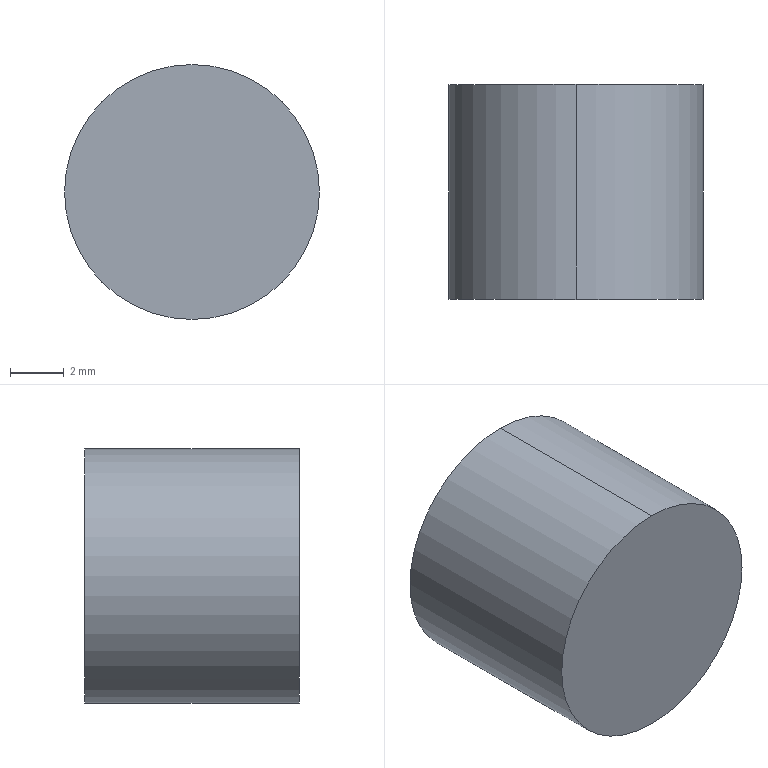Part | STEP file | 1-branch plug | 1 solid | 17 faces | box 9.5 x 8 x 9.5 mm | volume 424.158 mm3 | plane 15 | cylinder 2 | commonest cylinder face diameters 9.5 x2
STEP:
#1=CARTESIAN_POINT('',(0.,0.,0.));
#2=DIRECTION('',(0.,0.,1.));
#3=DIRECTION('',(1.,0.,0.));
#4=AXIS2_PLACEMENT_3D('',#1,#2,#3);
#5=CARTESIAN_POINT('',(0.,8.,4.75));
#6=VERTEX_POINT('',#5);
#7=CARTESIAN_POINT('',(0.,8.,-4.75));
#8=VERTEX_POINT('',#7);
#9=CARTESIAN_POINT('',(0.,8.,0.));
#10=DIRECTION('',(0.,1.,0.));
#11=DIRECTION('',(0.,0.,1.));
#12=AXIS2_PLACEMENT_3D('',#9,#10,#11);
#13=CIRCLE('',#12,4.75);
#14=CARTESIAN_POINT('',(0.,8.,0.));
#15=DIRECTION('',(0.,-1.,0.));
#16=DIRECTION('',(0.,0.,-1.));
#17=AXIS2_PLACEMENT_3D('',#14,#15,#16);
#18=CYLINDRICAL_SURFACE('',#17,4.75);
#19=CARTESIAN_POINT('',(3.142,0.));
#20=DIRECTION('',(-1.,0.));
#21=VECTOR('',#20,1.);
#22=LINE('',#19,#21);
#23=(GEOMETRIC_REPRESENTATION_CONTEXT(2)PARAMETRIC_REPRESENTATION_CONTEXT()REPRESENTATION_CONTEXT('',''));
#24=DEFINITIONAL_REPRESENTATION('',(#22),#23);
#25=PCURVE('',#18,#24);
#26=CARTESIAN_POINT('',(0.,8.,0.));
#27=DIRECTION('',(0.,1.,0.));
#28=DIRECTION('',(0.,0.,1.));
#29=AXIS2_PLACEMENT_3D('',#26,#27,#28);
#30=PLANE('',#29);
#31=CARTESIAN_POINT('',(0.,0.));
#32=DIRECTION('',(1.,0.));
#33=AXIS2_PLACEMENT_2D('',#31,#32);
#34=CIRCLE('',#33,4.75);
#35=(GEOMETRIC_REPRESENTATION_CONTEXT(2)PARAMETRIC_REPRESENTATION_CONTEXT()REPRESENTATION_CONTEXT('',''));
#36=DEFINITIONAL_REPRESENTATION('',(#34),#35);
#37=PCURVE('',#30,#36);
#38=SURFACE_CURVE('',#13,(#25,#37),.PCURVE_S1.);
#39=EDGE_CURVE('',#6,#8,#38,.T.);
#40=ORIENTED_EDGE('',*,*,#39,.F.);
#41=CARTESIAN_POINT('',(0.,0.,4.75));
#42=VERTEX_POINT('',#41);
#43=CARTESIAN_POINT('',(0.,8.,4.75));
#44=DIRECTION('',(0.,-1.,0.));
#45=VECTOR('',#44,1.);
#46=LINE('',#43,#45);
#47=CARTESIAN_POINT('',(3.142,0.));
#48=DIRECTION('',(0.,1.));
#49=VECTOR('',#48,1.);
#50=LINE('',#47,#49);
#51=(GEOMETRIC_REPRESENTATION_CONTEXT(2)PARAMETRIC_REPRESENTATION_CONTEXT()REPRESENTATION_CONTEXT('',''));
#52=DEFINITIONAL_REPRESENTATION('',(#50),#51);
#53=PCURVE('',#18,#52);
#54=CARTESIAN_POINT('',(0.,8.,0.));
#55=DIRECTION('',(0.,-1.,0.));
#56=DIRECTION('',(0.,0.,-1.));
#57=AXIS2_PLACEMENT_3D('',#54,#55,#56);
#58=CYLINDRICAL_SURFACE('',#57,4.75);
#59=CARTESIAN_POINT('',(3.142,0.));
#60=DIRECTION('',(0.,1.));
#61=VECTOR('',#60,1.);
#62=LINE('',#59,#61);
#63=(GEOMETRIC_REPRESENTATION_CONTEXT(2)PARAMETRIC_REPRESENTATION_CONTEXT()REPRESENTATION_CONTEXT('',''));
#64=DEFINITIONAL_REPRESENTATION('',(#62),#63);
#65=PCURVE('',#58,#64);
#66=SURFACE_CURVE('',#46,(#53,#65),.PCURVE_S1.);
#67=EDGE_CURVE('',#6,#42,#66,.T.);
#68=ORIENTED_EDGE('',*,*,#67,.T.);
#69=CARTESIAN_POINT('',(0.,0.,-4.75));
#70=VERTEX_POINT('',#69);
#71=CARTESIAN_POINT('',(0.,0.,0.));
#72=DIRECTION('',(0.,1.,0.));
#73=DIRECTION('',(0.,0.,1.));
#74=AXIS2_PLACEMENT_3D('',#71,#72,#73);
#75=CIRCLE('',#74,4.75);
#76=CARTESIAN_POINT('',(3.142,8.));
#77=DIRECTION('',(-1.,0.));
#78=VECTOR('',#77,1.);
#79=LINE('',#76,#78);
#80=(GEOMETRIC_REPRESENTATION_CONTEXT(2)PARAMETRIC_REPRESENTATION_CONTEXT()REPRESENTATION_CONTEXT('',''));
#81=DEFINITIONAL_REPRESENTATION('',(#79),#80);
#82=PCURVE('',#18,#81);
#83=CARTESIAN_POINT('',(0.,0.,0.));
#84=DIRECTION('',(0.,1.,0.));
#85=DIRECTION('',(0.,0.,1.));
#86=AXIS2_PLACEMENT_3D('',#83,#84,#85);
#87=PLANE('',#86);
#88=CARTESIAN_POINT('',(0.,0.));
#89=DIRECTION('',(1.,0.));
#90=AXIS2_PLACEMENT_2D('',#88,#89);
#91=CIRCLE('',#90,4.75);
#92=(GEOMETRIC_REPRESENTATION_CONTEXT(2)PARAMETRIC_REPRESENTATION_CONTEXT()REPRESENTATION_CONTEXT('',''));
#93=DEFINITIONAL_REPRESENTATION('',(#91),#92);
#94=PCURVE('',#87,#93);
#95=SURFACE_CURVE('',#75,(#82,#94),.PCURVE_S1.);
#96=EDGE_CURVE('',#42,#70,#95,.T.);
#97=ORIENTED_EDGE('',*,*,#96,.T.);
#98=CARTESIAN_POINT('',(0.,8.,-4.75));
#99=DIRECTION('',(0.,-1.,0.));
#100=VECTOR('',#99,1.);
#101=LINE('',#98,#100);
#102=CARTESIAN_POINT('',(0.,0.));
#103=DIRECTION('',(0.,1.));
#104=VECTOR('',#103,1.);
#105=LINE('',#102,#104);
#106=(GEOMETRIC_REPRESENTATION_CONTEXT(2)PARAMETRIC_REPRESENTATION_CONTEXT()REPRESENTATION_CONTEXT('',''));
#107=DEFINITIONAL_REPRESENTATION('',(#105),#106);
#108=PCURVE('',#18,#107);
#109=CARTESIAN_POINT('',(6.283,0.));
#110=DIRECTION('',(0.,1.));
#111=VECTOR('',#110,1.);
#112=LINE('',#109,#111);
#113=(GEOMETRIC_REPRESENTATION_CONTEXT(2)PARAMETRIC_REPRESENTATION_CONTEXT()REPRESENTATION_CONTEXT('',''));
#114=DEFINITIONAL_REPRESENTATION('',(#112),#113);
#115=PCURVE('',#58,#114);
#116=SURFACE_CURVE('',#101,(#108,#115),.PCURVE_S1.);
#117=EDGE_CURVE('',#8,#70,#116,.T.);
#118=ORIENTED_EDGE('',*,*,#117,.F.);
#119=EDGE_LOOP('',(#40,#68,#97,#118));
#120=FACE_BOUND('',#119,.T.);
#121=ADVANCED_FACE('',(#120),#18,.T.);
#122=ORIENTED_EDGE('',*,*,#67,.F.);
#123=CARTESIAN_POINT('',(0.,8.,0.));
#124=DIRECTION('',(0.,1.,0.));
#125=DIRECTION('',(0.,0.,1.));
#126=AXIS2_PLACEMENT_3D('',#123,#124,#125);
#127=CIRCLE('',#126,4.75);
#128=CARTESIAN_POINT('',(9.425,0.));
#129=DIRECTION('',(-1.,0.));
#130=VECTOR('',#129,1.);
#131=LINE('',#128,#130);
#132=(GEOMETRIC_REPRESENTATION_CONTEXT(2)PARAMETRIC_REPRESENTATION_CONTEXT()REPRESENTATION_CONTEXT('',''));
#133=DEFINITIONAL_REPRESENTATION('',(#131),#132);
#134=PCURVE('',#58,#133);
#135=CARTESIAN_POINT('',(0.,0.));
#136=DIRECTION('',(1.,0.));
#137=AXIS2_PLACEMENT_2D('',#135,#136);
#138=CIRCLE('',#137,4.75);
#139=(GEOMETRIC_REPRESENTATION_CONTEXT(2)PARAMETRIC_REPRESENTATION_CONTEXT()REPRESENTATION_CONTEXT('',''));
#140=DEFINITIONAL_REPRESENTATION('',(#138),#139);
#141=PCURVE('',#30,#140);
#142=SURFACE_CURVE('',#127,(#134,#141),.PCURVE_S1.);
#143=EDGE_CURVE('',#8,#6,#142,.T.);
#144=ORIENTED_EDGE('',*,*,#143,.F.);
#145=ORIENTED_EDGE('',*,*,#117,.T.);
#146=CARTESIAN_POINT('',(0.,0.,0.));
#147=DIRECTION('',(0.,1.,0.));
#148=DIRECTION('',(0.,0.,1.));
#149=AXIS2_PLACEMENT_3D('',#146,#147,#148);
#150=CIRCLE('',#149,4.75);
#151=CARTESIAN_POINT('',(9.425,8.));
#152=DIRECTION('',(-1.,0.));
#153=VECTOR('',#152,1.);
#154=LINE('',#151,#153);
#155=(GEOMETRIC_REPRESENTATION_CONTEXT(2)PARAMETRIC_REPRESENTATION_CONTEXT()REPRESENTATION_CONTEXT('',''));
#156=DEFINITIONAL_REPRESENTATION('',(#154),#155);
#157=PCURVE('',#58,#156);
#158=CARTESIAN_POINT('',(0.,0.));
#159=DIRECTION('',(1.,0.));
#160=AXIS2_PLACEMENT_2D('',#158,#159);
#161=CIRCLE('',#160,4.75);
#162=(GEOMETRIC_REPRESENTATION_CONTEXT(2)PARAMETRIC_REPRESENTATION_CONTEXT()REPRESENTATION_CONTEXT('',''));
#163=DEFINITIONAL_REPRESENTATION('',(#161),#162);
#164=PCURVE('',#87,#163);
#165=SURFACE_CURVE('',#150,(#157,#164),.PCURVE_S1.);
#166=EDGE_CURVE('',#70,#42,#165,.T.);
#167=ORIENTED_EDGE('',*,*,#166,.T.);
#168=EDGE_LOOP('',(#122,#144,#145,#167));
#169=FACE_BOUND('',#168,.T.);
#170=ADVANCED_FACE('',(#169),#58,.T.);
#171=CARTESIAN_POINT('',(-3.579,8.,0.04065));
#172=VERTEX_POINT('',#171);
#173=CARTESIAN_POINT('',(-1.825,8.,-3.079));
#174=VERTEX_POINT('',#173);
#175=CARTESIAN_POINT('',(-1.966,8.,-2.828));
#176=DIRECTION('',(0.4901,0.,-0.8716));
#177=VECTOR('',#176,1.);
#178=LINE('',#175,#177);
#179=CARTESIAN_POINT('',(-2.828,-1.966));
#180=DIRECTION('',(-0.8716,0.4901));
#181=VECTOR('',#180,1.);
#182=LINE('',#179,#181);
#183=(GEOMETRIC_REPRESENTATION_CONTEXT(2)PARAMETRIC_REPRESENTATION_CONTEXT()REPRESENTATION_CONTEXT('',''));
#184=DEFINITIONAL_REPRESENTATION('',(#182),#183);
#185=PCURVE('',#30,#184);
#186=CARTESIAN_POINT('',(-1.531,7.5,-2.583));
#187=DIRECTION('',(0.6163,0.7071,0.3466));
#188=DIRECTION('',(0.4901,0.,-0.8716));
#189=AXIS2_PLACEMENT_3D('',#186,#187,#188);
#190=PLANE('',#189);
#191=CARTESIAN_POINT('',(0.,0.7071));
#192=DIRECTION('',(1.,0.));
#193=VECTOR('',#192,1.);
#194=LINE('',#191,#193);
#195=(GEOMETRIC_REPRESENTATION_CONTEXT(2)PARAMETRIC_REPRESENTATION_CONTEXT()REPRESENTATION_CONTEXT('',''));
#196=DEFINITIONAL_REPRESENTATION('',(#194),#195);
#197=PCURVE('',#190,#196);
#198=SURFACE_CURVE('',#178,(#185,#197),.PCURVE_S1.);
#199=EDGE_CURVE('',#172,#174,#198,.T.);
#200=ORIENTED_EDGE('',*,*,#199,.T.);
#201=CARTESIAN_POINT('',(1.754,8.,-3.12));
#202=VERTEX_POINT('',#201);
#203=CARTESIAN_POINT('',(1.466,8.,-3.117));
#204=DIRECTION('',(0.9999,0.,-0.01136));
#205=VECTOR('',#204,1.);
#206=LINE('',#203,#205);
#207=CARTESIAN_POINT('',(-3.117,1.466));
#208=DIRECTION('',(-0.01136,0.9999));
#209=VECTOR('',#208,1.);
#210=LINE('',#207,#209);
#211=(GEOMETRIC_REPRESENTATION_CONTEXT(2)PARAMETRIC_REPRESENTATION_CONTEXT()REPRESENTATION_CONTEXT('',''));
#212=DEFINITIONAL_REPRESENTATION('',(#210),#211);
#213=PCURVE('',#30,#212);
#214=CARTESIAN_POINT('',(1.471,7.5,-2.617));
#215=DIRECTION('',(0.00803,0.7071,0.7071));
#216=DIRECTION('',(0.9999,0.,-0.01136));
#217=AXIS2_PLACEMENT_3D('',#214,#215,#216);
#218=PLANE('',#217);
#219=CARTESIAN_POINT('',(0.,0.7071));
#220=DIRECTION('',(1.,0.));
#221=VECTOR('',#220,1.);
#222=LINE('',#219,#221);
#223=(GEOMETRIC_REPRESENTATION_CONTEXT(2)PARAMETRIC_REPRESENTATION_CONTEXT()REPRESENTATION_CONTEXT('',''));
#224=DEFINITIONAL_REPRESENTATION('',(#222),#223);
#225=PCURVE('',#218,#224);
#226=SURFACE_CURVE('',#206,(#213,#225),.PCURVE_S1.);
#227=EDGE_CURVE('',#174,#202,#226,.T.);
#228=ORIENTED_EDGE('',*,*,#227,.T.);
#229=CARTESIAN_POINT('',(3.579,8.,-0.04065));
#230=VERTEX_POINT('',#229);
#231=CARTESIAN_POINT('',(3.432,8.,-0.289));
#232=DIRECTION('',(0.5098,0.,0.8603));
#233=VECTOR('',#232,1.);
#234=LINE('',#231,#233);
#235=CARTESIAN_POINT('',(-0.289,3.432));
#236=DIRECTION('',(0.8603,0.5098));
#237=VECTOR('',#236,1.);
#238=LINE('',#235,#237);
#239=(GEOMETRIC_REPRESENTATION_CONTEXT(2)PARAMETRIC_REPRESENTATION_CONTEXT()REPRESENTATION_CONTEXT('',''));
#240=DEFINITIONAL_REPRESENTATION('',(#238),#239);
#241=PCURVE('',#30,#240);
#242=CARTESIAN_POINT('',(3.002,7.5,-0.03409));
#243=DIRECTION('',(-0.6083,0.7071,0.3605));
#244=DIRECTION('',(0.5098,0.,0.8603));
#245=AXIS2_PLACEMENT_3D('',#242,#243,#244);
#246=PLANE('',#245);
#247=CARTESIAN_POINT('',(0.,0.7071));
#248=DIRECTION('',(1.,0.));
#249=VECTOR('',#248,1.);
#250=LINE('',#247,#249);
#251=(GEOMETRIC_REPRESENTATION_CONTEXT(2)PARAMETRIC_REPRESENTATION_CONTEXT()REPRESENTATION_CONTEXT('',''));
#252=DEFINITIONAL_REPRESENTATION('',(#250),#251);
#253=PCURVE('',#246,#252);
#254=SURFACE_CURVE('',#234,(#241,#253),.PCURVE_S1.);
#255=EDGE_CURVE('',#202,#230,#254,.T.);
#256=ORIENTED_EDGE('',*,*,#255,.T.);
#257=CARTESIAN_POINT('',(1.825,8.,3.079));
#258=VERTEX_POINT('',#257);
#259=CARTESIAN_POINT('',(1.966,8.,2.828));
#260=DIRECTION('',(-0.4901,0.,0.8716));
#261=VECTOR('',#260,1.);
#262=LINE('',#259,#261);
#263=CARTESIAN_POINT('',(2.828,1.966));
#264=DIRECTION('',(0.8716,-0.4901));
#265=VECTOR('',#264,1.);
#266=LINE('',#263,#265);
#267=(GEOMETRIC_REPRESENTATION_CONTEXT(2)PARAMETRIC_REPRESENTATION_CONTEXT()REPRESENTATION_CONTEXT('',''));
#268=DEFINITIONAL_REPRESENTATION('',(#266),#267);
#269=PCURVE('',#30,#268);
#270=CARTESIAN_POINT('',(1.531,7.5,2.583));
#271=DIRECTION('',(-0.6163,0.7071,-0.3466));
#272=DIRECTION('',(-0.4901,0.,0.8716));
#273=AXIS2_PLACEMENT_3D('',#270,#271,#272);
#274=PLANE('',#273);
#275=CARTESIAN_POINT('',(0.,0.7071));
#276=DIRECTION('',(1.,0.));
#277=VECTOR('',#276,1.);
#278=LINE('',#275,#277);
#279=(GEOMETRIC_REPRESENTATION_CONTEXT(2)PARAMETRIC_REPRESENTATION_CONTEXT()REPRESENTATION_CONTEXT('',''));
#280=DEFINITIONAL_REPRESENTATION('',(#278),#279);
#281=PCURVE('',#274,#280);
#282=SURFACE_CURVE('',#262,(#269,#281),.PCURVE_S1.);
#283=EDGE_CURVE('',#230,#258,#282,.T.);
#284=ORIENTED_EDGE('',*,*,#283,.T.);
#285=CARTESIAN_POINT('',(-1.754,8.,3.12));
#286=VERTEX_POINT('',#285);
#287=CARTESIAN_POINT('',(-1.466,8.,3.117));
#288=DIRECTION('',(-0.9999,0.,0.01136));
#289=VECTOR('',#288,1.);
#290=LINE('',#287,#289);
#291=CARTESIAN_POINT('',(3.117,-1.466));
#292=DIRECTION('',(0.01136,-0.9999));
#293=VECTOR('',#292,1.);
#294=LINE('',#291,#293);
#295=(GEOMETRIC_REPRESENTATION_CONTEXT(2)PARAMETRIC_REPRESENTATION_CONTEXT()REPRESENTATION_CONTEXT('',''));
#296=DEFINITIONAL_REPRESENTATION('',(#294),#295);
#297=PCURVE('',#30,#296);
#298=CARTESIAN_POINT('',(-1.471,7.5,2.617));
#299=DIRECTION('',(-0.00803,0.7071,-0.7071));
#300=DIRECTION('',(-0.9999,0.,0.01136));
#301=AXIS2_PLACEMENT_3D('',#298,#299,#300);
#302=PLANE('',#301);
#303=CARTESIAN_POINT('',(0.,0.7071));
#304=DIRECTION('',(1.,0.));
#305=VECTOR('',#304,1.);
#306=LINE('',#303,#305);
#307=(GEOMETRIC_REPRESENTATION_CONTEXT(2)PARAMETRIC_REPRESENTATION_CONTEXT()REPRESENTATION_CONTEXT('',''));
#308=DEFINITIONAL_REPRESENTATION('',(#306),#307);
#309=PCURVE('',#302,#308);
#310=SURFACE_CURVE('',#290,(#297,#309),.PCURVE_S1.);
#311=EDGE_CURVE('',#258,#286,#310,.T.);
#312=ORIENTED_EDGE('',*,*,#311,.T.);
#313=CARTESIAN_POINT('',(-3.432,8.,0.289));
#314=DIRECTION('',(-0.5098,0.,-0.8603));
#315=VECTOR('',#314,1.);
#316=LINE('',#313,#315);
#317=CARTESIAN_POINT('',(0.289,-3.432));
#318=DIRECTION('',(-0.8603,-0.5098));
#319=VECTOR('',#318,1.);
#320=LINE('',#317,#319);
#321=(GEOMETRIC_REPRESENTATION_CONTEXT(2)PARAMETRIC_REPRESENTATION_CONTEXT()REPRESENTATION_CONTEXT('',''));
#322=DEFINITIONAL_REPRESENTATION('',(#320),#321);
#323=PCURVE('',#30,#322);
#324=CARTESIAN_POINT('',(-3.002,7.5,0.03409));
#325=DIRECTION('',(0.6083,0.7071,-0.3605));
#326=DIRECTION('',(-0.5098,0.,-0.8603));
#327=AXIS2_PLACEMENT_3D('',#324,#325,#326);
#328=PLANE('',#327);
#329=CARTESIAN_POINT('',(0.,0.7071));
#330=DIRECTION('',(1.,0.));
#331=VECTOR('',#330,1.);
#332=LINE('',#329,#331);
#333=(GEOMETRIC_REPRESENTATION_CONTEXT(2)PARAMETRIC_REPRESENTATION_CONTEXT()REPRESENTATION_CONTEXT('',''));
#334=DEFINITIONAL_REPRESENTATION('',(#332),#333);
#335=PCURVE('',#328,#334);
#336=SURFACE_CURVE('',#316,(#323,#335),.PCURVE_S1.);
#337=EDGE_CURVE('',#286,#172,#336,.T.);
#338=ORIENTED_EDGE('',*,*,#337,.T.);
#339=EDGE_LOOP('',(#200,#228,#256,#284,#312,#338));
#340=FACE_BOUND('',#339,.T.);
#341=ORIENTED_EDGE('',*,*,#143,.T.);
#342=ORIENTED_EDGE('',*,*,#39,.T.);
#343=EDGE_LOOP('',(#341,#342));
#344=FACE_BOUND('',#343,.T.);
#345=ADVANCED_FACE('',(#340,#344),#30,.T.);
#346=ORIENTED_EDGE('',*,*,#166,.F.);
#347=ORIENTED_EDGE('',*,*,#96,.F.);
#348=EDGE_LOOP('',(#346,#347));
#349=FACE_BOUND('',#348,.T.);
#350=ADVANCED_FACE('',(#349),#87,.F.);
#351=CARTESIAN_POINT('',(-1.471,2.,2.617));
#352=VERTEX_POINT('',#351);
#353=CARTESIAN_POINT('',(-1.471,7.5,2.617));
#354=VERTEX_POINT('',#353);
#355=CARTESIAN_POINT('',(-1.471,2.,2.617));
#356=DIRECTION('',(0.,1.,0.));
#357=VECTOR('',#356,1.);
#358=LINE('',#355,#357);
#359=CARTESIAN_POINT('',(-1.471,2.,2.617));
#360=DIRECTION('',(0.01136,0.,0.9999));
#361=DIRECTION('',(0.9999,0.,-0.01136));
#362=AXIS2_PLACEMENT_3D('',#359,#360,#361);
#363=PLANE('',#362);
#364=CARTESIAN_POINT('',(0.,0.));
#365=DIRECTION('',(0.,1.));
#366=VECTOR('',#365,1.);
#367=LINE('',#364,#366);
#368=(GEOMETRIC_REPRESENTATION_CONTEXT(2)PARAMETRIC_REPRESENTATION_CONTEXT()REPRESENTATION_CONTEXT('',''));
#369=DEFINITIONAL_REPRESENTATION('',(#367),#368);
#370=PCURVE('',#363,#369);
#371=CARTESIAN_POINT('',(-3.002,2.,0.03409));
#372=DIRECTION('',(-0.8603,0.,0.5098));
#373=DIRECTION('',(0.5098,0.,0.8603));
#374=AXIS2_PLACEMENT_3D('',#371,#372,#373);
#375=PLANE('',#374);
#376=CARTESIAN_POINT('',(3.002,0.));
#377=DIRECTION('',(0.,1.));
#378=VECTOR('',#377,1.);
#379=LINE('',#376,#378);
#380=(GEOMETRIC_REPRESENTATION_CONTEXT(2)PARAMETRIC_REPRESENTATION_CONTEXT()REPRESENTATION_CONTEXT('',''));
#381=DEFINITIONAL_REPRESENTATION('',(#379),#380);
#382=PCURVE('',#375,#381);
#383=SURFACE_CURVE('',#358,(#370,#382),.PCURVE_S1.);
#384=EDGE_CURVE('',#352,#354,#383,.T.);
#385=ORIENTED_EDGE('',*,*,#384,.T.);
#386=CARTESIAN_POINT('',(1.531,7.5,2.583));
#387=VERTEX_POINT('',#386);
#388=CARTESIAN_POINT('',(1.531,7.5,2.583));
#389=DIRECTION('',(0.9999,0.,-0.01136));
#390=VECTOR('',#389,1.);
#391=LINE('',#388,#390);
#392=CARTESIAN_POINT('',(3.002,5.5));
#393=DIRECTION('',(1.,0.));
#394=VECTOR('',#393,1.);
#395=LINE('',#392,#394);
#396=(GEOMETRIC_REPRESENTATION_CONTEXT(2)PARAMETRIC_REPRESENTATION_CONTEXT()REPRESENTATION_CONTEXT('',''));
#397=DEFINITIONAL_REPRESENTATION('',(#395),#396);
#398=PCURVE('',#363,#397);
#399=CARTESIAN_POINT('',(-3.002,0.));
#400=DIRECTION('',(-1.,0.));
#401=VECTOR('',#400,1.);
#402=LINE('',#399,#401);
#403=(GEOMETRIC_REPRESENTATION_CONTEXT(2)PARAMETRIC_REPRESENTATION_CONTEXT()REPRESENTATION_CONTEXT('',''));
#404=DEFINITIONAL_REPRESENTATION('',(#402),#403);
#405=PCURVE('',#302,#404);
#406=SURFACE_CURVE('',#391,(#398,#405),.PCURVE_S1.);
#407=EDGE_CURVE('',#354,#387,#406,.T.);
#408=ORIENTED_EDGE('',*,*,#407,.T.);
#409=CARTESIAN_POINT('',(1.531,2.,2.583));
#410=VERTEX_POINT('',#409);
#411=CARTESIAN_POINT('',(1.531,2.,2.583));
#412=DIRECTION('',(0.,1.,0.));
#413=VECTOR('',#412,1.);
#414=LINE('',#411,#413);
#415=CARTESIAN_POINT('',(3.002,0.));
#416=DIRECTION('',(0.,1.));
#417=VECTOR('',#416,1.);
#418=LINE('',#415,#417);
#419=(GEOMETRIC_REPRESENTATION_CONTEXT(2)PARAMETRIC_REPRESENTATION_CONTEXT()REPRESENTATION_CONTEXT('',''));
#420=DEFINITIONAL_REPRESENTATION('',(#418),#419);
#421=PCURVE('',#363,#420);
#422=CARTESIAN_POINT('',(1.531,2.,2.583));
#423=DIRECTION('',(0.8716,0.,0.4901));
#424=DIRECTION('',(0.4901,0.,-0.8716));
#425=AXIS2_PLACEMENT_3D('',#422,#423,#424);
#426=PLANE('',#425);
#427=CARTESIAN_POINT('',(0.,0.));
#428=DIRECTION('',(0.,1.));
#429=VECTOR('',#428,1.);
#430=LINE('',#427,#429);
#431=(GEOMETRIC_REPRESENTATION_CONTEXT(2)PARAMETRIC_REPRESENTATION_CONTEXT()REPRESENTATION_CONTEXT('',''));
#432=DEFINITIONAL_REPRESENTATION('',(#430),#431);
#433=PCURVE('',#426,#432);
#434=SURFACE_CURVE('',#414,(#421,#433),.PCURVE_S1.);
#435=EDGE_CURVE('',#410,#387,#434,.T.);
#436=ORIENTED_EDGE('',*,*,#435,.F.);
#437=CARTESIAN_POINT('',(-1.471,2.,2.617));
#438=DIRECTION('',(0.9999,0.,-0.01136));
#439=VECTOR('',#438,1.);
#440=LINE('',#437,#439);
#441=CARTESIAN_POINT('',(0.,0.));
#442=DIRECTION('',(1.,0.));
#443=VECTOR('',#442,1.);
#444=LINE('',#441,#443);
#445=(GEOMETRIC_REPRESENTATION_CONTEXT(2)PARAMETRIC_REPRESENTATION_CONTEXT()REPRESENTATION_CONTEXT('',''));
#446=DEFINITIONAL_REPRESENTATION('',(#444),#445);
#447=PCURVE('',#363,#446);
#448=CARTESIAN_POINT('',(0.,2.,0.));
#449=DIRECTION('',(0.,1.,0.));
#450=DIRECTION('',(0.,0.,1.));
#451=AXIS2_PLACEMENT_3D('',#448,#449,#450);
#452=PLANE('',#451);
#453=CARTESIAN_POINT('',(2.617,-1.471));
#454=DIRECTION('',(-0.01136,0.9999));
#455=VECTOR('',#454,1.);
#456=LINE('',#453,#455);
#457=(GEOMETRIC_REPRESENTATION_CONTEXT(2)PARAMETRIC_REPRESENTATION_CONTEXT()REPRESENTATION_CONTEXT('',''));
#458=DEFINITIONAL_REPRESENTATION('',(#456),#457);
#459=PCURVE('',#452,#458);
#460=SURFACE_CURVE('',#440,(#447,#459),.PCURVE_S1.);
#461=EDGE_CURVE('',#352,#410,#460,.T.);
#462=ORIENTED_EDGE('',*,*,#461,.F.);
#463=EDGE_LOOP('',(#385,#408,#436,#462));
#464=FACE_BOUND('',#463,.T.);
#465=ADVANCED_FACE('',(#464),#363,.F.);
#466=CARTESIAN_POINT('',(-3.002,2.,0.03409));
#467=VERTEX_POINT('',#466);
#468=CARTESIAN_POINT('',(-3.002,7.5,0.03409));
#469=VERTEX_POINT('',#468);
#470=CARTESIAN_POINT('',(-3.002,2.,0.03409));
#471=DIRECTION('',(0.,1.,0.));
#472=VECTOR('',#471,1.);
#473=LINE('',#470,#472);
#474=CARTESIAN_POINT('',(0.,0.));
#475=DIRECTION('',(0.,1.));
#476=VECTOR('',#475,1.);
#477=LINE('',#474,#476);
#478=(GEOMETRIC_REPRESENTATION_CONTEXT(2)PARAMETRIC_REPRESENTATION_CONTEXT()REPRESENTATION_CONTEXT('',''));
#479=DEFINITIONAL_REPRESENTATION('',(#477),#478);
#480=PCURVE('',#375,#479);
#481=CARTESIAN_POINT('',(-1.531,2.,-2.583));
#482=DIRECTION('',(-0.8716,0.,-0.4901));
#483=DIRECTION('',(-0.4901,0.,0.8716));
#484=AXIS2_PLACEMENT_3D('',#481,#482,#483);
#485=PLANE('',#484);
#486=CARTESIAN_POINT('',(3.002,0.));
#487=DIRECTION('',(0.,1.));
#488=VECTOR('',#487,1.);
#489=LINE('',#486,#488);
#490=(GEOMETRIC_REPRESENTATION_CONTEXT(2)PARAMETRIC_REPRESENTATION_CONTEXT()REPRESENTATION_CONTEXT('',''));
#491=DEFINITIONAL_REPRESENTATION('',(#489),#490);
#492=PCURVE('',#485,#491);
#493=SURFACE_CURVE('',#473,(#480,#492),.PCURVE_S1.);
#494=EDGE_CURVE('',#467,#469,#493,.T.);
#495=ORIENTED_EDGE('',*,*,#494,.T.);
#496=CARTESIAN_POINT('',(-1.471,7.5,2.617));
#497=DIRECTION('',(0.5098,0.,0.8603));
#498=VECTOR('',#497,1.);
#499=LINE('',#496,#498);
#500=CARTESIAN_POINT('',(3.002,5.5));
#501=DIRECTION('',(1.,0.));
#502=VECTOR('',#501,1.);
#503=LINE('',#500,#502);
#504=(GEOMETRIC_REPRESENTATION_CONTEXT(2)PARAMETRIC_REPRESENTATION_CONTEXT()REPRESENTATION_CONTEXT('',''));
#505=DEFINITIONAL_REPRESENTATION('',(#503),#504);
#506=PCURVE('',#375,#505);
#507=CARTESIAN_POINT('',(-3.002,0.));
#508=DIRECTION('',(-1.,0.));
#509=VECTOR('',#508,1.);
#510=LINE('',#507,#509);
#511=(GEOMETRIC_REPRESENTATION_CONTEXT(2)PARAMETRIC_REPRESENTATION_CONTEXT()REPRESENTATION_CONTEXT('',''));
#512=DEFINITIONAL_REPRESENTATION('',(#510),#511);
#513=PCURVE('',#328,#512);
#514=SURFACE_CURVE('',#499,(#506,#513),.PCURVE_S1.);
#515=EDGE_CURVE('',#469,#354,#514,.T.);
#516=ORIENTED_EDGE('',*,*,#515,.T.);
#517=ORIENTED_EDGE('',*,*,#384,.F.);
#518=CARTESIAN_POINT('',(-3.002,2.,0.03409));
#519=DIRECTION('',(0.5098,0.,0.8603));
#520=VECTOR('',#519,1.);
#521=LINE('',#518,#520);
#522=CARTESIAN_POINT('',(0.,0.));
#523=DIRECTION('',(1.,0.));
#524=VECTOR('',#523,1.);
#525=LINE('',#522,#524);
#526=(GEOMETRIC_REPRESENTATION_CONTEXT(2)PARAMETRIC_REPRESENTATION_CONTEXT()REPRESENTATION_CONTEXT('',''));
#527=DEFINITIONAL_REPRESENTATION('',(#525),#526);
#528=PCURVE('',#375,#527);
#529=CARTESIAN_POINT('',(0.03409,-3.002));
#530=DIRECTION('',(0.8603,0.5098));
#531=VECTOR('',#530,1.);
#532=LINE('',#529,#531);
#533=(GEOMETRIC_REPRESENTATION_CONTEXT(2)PARAMETRIC_REPRESENTATION_CONTEXT()REPRESENTATION_CONTEXT('',''));
#534=DEFINITIONAL_REPRESENTATION('',(#532),#533);
#535=PCURVE('',#452,#534);
#536=SURFACE_CURVE('',#521,(#528,#535),.PCURVE_S1.);
#537=EDGE_CURVE('',#467,#352,#536,.T.);
#538=ORIENTED_EDGE('',*,*,#537,.F.);
#539=EDGE_LOOP('',(#495,#516,#517,#538));
#540=FACE_BOUND('',#539,.T.);
#541=ADVANCED_FACE('',(#540),#375,.F.);
#542=CARTESIAN_POINT('',(-1.531,2.,-2.583));
#543=VERTEX_POINT('',#542);
#544=CARTESIAN_POINT('',(-1.531,7.5,-2.583));
#545=VERTEX_POINT('',#544);
#546=CARTESIAN_POINT('',(-1.531,2.,-2.583));
#547=DIRECTION('',(0.,1.,0.));
#548=VECTOR('',#547,1.);
#549=LINE('',#546,#548);
#550=CARTESIAN_POINT('',(0.,0.));
#551=DIRECTION('',(0.,1.));
#552=VECTOR('',#551,1.);
#553=LINE('',#550,#552);
#554=(GEOMETRIC_REPRESENTATION_CONTEXT(2)PARAMETRIC_REPRESENTATION_CONTEXT()REPRESENTATION_CONTEXT('',''));
#555=DEFINITIONAL_REPRESENTATION('',(#553),#554);
#556=PCURVE('',#485,#555);
#557=CARTESIAN_POINT('',(1.471,2.,-2.617));
#558=DIRECTION('',(-0.01136,0.,-0.9999));
#559=DIRECTION('',(-0.9999,0.,0.01136));
#560=AXIS2_PLACEMENT_3D('',#557,#558,#559);
#561=PLANE('',#560);
#562=CARTESIAN_POINT('',(3.002,0.));
#563=DIRECTION('',(0.,1.));
#564=VECTOR('',#563,1.);
#565=LINE('',#562,#564);
#566=(GEOMETRIC_REPRESENTATION_CONTEXT(2)PARAMETRIC_REPRESENTATION_CONTEXT()REPRESENTATION_CONTEXT('',''));
#567=DEFINITIONAL_REPRESENTATION('',(#565),#566);
#568=PCURVE('',#561,#567);
#569=SURFACE_CURVE('',#549,(#556,#568),.PCURVE_S1.);
#570=EDGE_CURVE('',#543,#545,#569,.T.);
#571=ORIENTED_EDGE('',*,*,#570,.T.);
#572=CARTESIAN_POINT('',(-3.002,7.5,0.03409));
#573=DIRECTION('',(-0.4901,0.,0.8716));
#574=VECTOR('',#573,1.);
#575=LINE('',#572,#574);
#576=CARTESIAN_POINT('',(3.002,5.5));
#577=DIRECTION('',(1.,0.));
#578=VECTOR('',#577,1.);
#579=LINE('',#576,#578);
#580=(GEOMETRIC_REPRESENTATION_CONTEXT(2)PARAMETRIC_REPRESENTATION_CONTEXT()REPRESENTATION_CONTEXT('',''));
#581=DEFINITIONAL_REPRESENTATION('',(#579),#580);
#582=PCURVE('',#485,#581);
#583=CARTESIAN_POINT('',(-3.002,0.));
#584=DIRECTION('',(-1.,0.));
#585=VECTOR('',#584,1.);
#586=LINE('',#583,#585);
#587=(GEOMETRIC_REPRESENTATION_CONTEXT(2)PARAMETRIC_REPRESENTATION_CONTEXT()REPRESENTATION_CONTEXT('',''));
#588=DEFINITIONAL_REPRESENTATION('',(#586),#587);
#589=PCURVE('',#190,#588);
#590=SURFACE_CURVE('',#575,(#582,#589),.PCURVE_S1.);
#591=EDGE_CURVE('',#545,#469,#590,.T.);
#592=ORIENTED_EDGE('',*,*,#591,.T.);
#593=ORIENTED_EDGE('',*,*,#494,.F.);
#594=CARTESIAN_POINT('',(-1.531,2.,-2.583));
#595=DIRECTION('',(-0.4901,0.,0.8716));
#596=VECTOR('',#595,1.);
#597=LINE('',#594,#596);
#598=CARTESIAN_POINT('',(0.,0.));
#599=DIRECTION('',(1.,0.));
#600=VECTOR('',#599,1.);
#601=LINE('',#598,#600);
#602=(GEOMETRIC_REPRESENTATION_CONTEXT(2)PARAMETRIC_REPRESENTATION_CONTEXT()REPRESENTATION_CONTEXT('',''));
#603=DEFINITIONAL_REPRESENTATION('',(#601),#602);
#604=PCURVE('',#485,#603);
#605=CARTESIAN_POINT('',(-2.583,-1.531));
#606=DIRECTION('',(0.8716,-0.4901));
#607=VECTOR('',#606,1.);
#608=LINE('',#605,#607);
#609=(GEOMETRIC_REPRESENTATION_CONTEXT(2)PARAMETRIC_REPRESENTATION_CONTEXT()REPRESENTATION_CONTEXT('',''));
#610=DEFINITIONAL_REPRESENTATION('',(#608),#609);
#611=PCURVE('',#452,#610);
#612=SURFACE_CURVE('',#597,(#604,#611),.PCURVE_S1.);
#613=EDGE_CURVE('',#543,#467,#612,.T.);
#614=ORIENTED_EDGE('',*,*,#613,.F.);
#615=EDGE_LOOP('',(#571,#592,#593,#614));
#616=FACE_BOUND('',#615,.T.);
#617=ADVANCED_FACE('',(#616),#485,.F.);
#618=CARTESIAN_POINT('',(1.471,2.,-2.617));
#619=VERTEX_POINT('',#618);
#620=CARTESIAN_POINT('',(1.471,7.5,-2.617));
#621=VERTEX_POINT('',#620);
#622=CARTESIAN_POINT('',(1.471,2.,-2.617));
#623=DIRECTION('',(0.,1.,0.));
#624=VECTOR('',#623,1.);
#625=LINE('',#622,#624);
#626=CARTESIAN_POINT('',(0.,0.));
#627=DIRECTION('',(0.,1.));
#628=VECTOR('',#627,1.);
#629=LINE('',#626,#628);
#630=(GEOMETRIC_REPRESENTATION_CONTEXT(2)PARAMETRIC_REPRESENTATION_CONTEXT()REPRESENTATION_CONTEXT('',''));
#631=DEFINITIONAL_REPRESENTATION('',(#629),#630);
#632=PCURVE('',#561,#631);
#633=CARTESIAN_POINT('',(3.002,2.,-0.03409));
#634=DIRECTION('',(0.8603,0.,-0.5098));
#635=DIRECTION('',(-0.5098,0.,-0.8603));
#636=AXIS2_PLACEMENT_3D('',#633,#634,#635);
#637=PLANE('',#636);
#638=CARTESIAN_POINT('',(3.002,0.));
#639=DIRECTION('',(0.,1.));
#640=VECTOR('',#639,1.);
#641=LINE('',#638,#640);
#642=(GEOMETRIC_REPRESENTATION_CONTEXT(2)PARAMETRIC_REPRESENTATION_CONTEXT()REPRESENTATION_CONTEXT('',''));
#643=DEFINITIONAL_REPRESENTATION('',(#641),#642);
#644=PCURVE('',#637,#643);
#645=SURFACE_CURVE('',#625,(#632,#644),.PCURVE_S1.);
#646=EDGE_CURVE('',#619,#621,#645,.T.);
#647=ORIENTED_EDGE('',*,*,#646,.T.);
#648=CARTESIAN_POINT('',(-1.531,7.5,-2.583));
#649=DIRECTION('',(-0.9999,0.,0.01136));
#650=VECTOR('',#649,1.);
#651=LINE('',#648,#650);
#652=CARTESIAN_POINT('',(3.002,5.5));
#653=DIRECTION('',(1.,0.));
#654=VECTOR('',#653,1.);
#655=LINE('',#652,#654);
#656=(GEOMETRIC_REPRESENTATION_CONTEXT(2)PARAMETRIC_REPRESENTATION_CONTEXT()REPRESENTATION_CONTEXT('',''));
#657=DEFINITIONAL_REPRESENTATION('',(#655),#656);
#658=PCURVE('',#561,#657);
#659=CARTESIAN_POINT('',(-3.002,0.));
#660=DIRECTION('',(-1.,0.));
#661=VECTOR('',#660,1.);
#662=LINE('',#659,#661);
#663=(GEOMETRIC_REPRESENTATION_CONTEXT(2)PARAMETRIC_REPRESENTATION_CONTEXT()REPRESENTATION_CONTEXT('',''));
#664=DEFINITIONAL_REPRESENTATION('',(#662),#663);
#665=PCURVE('',#218,#664);
#666=SURFACE_CURVE('',#651,(#658,#665),.PCURVE_S1.);
#667=EDGE_CURVE('',#621,#545,#666,.T.);
#668=ORIENTED_EDGE('',*,*,#667,.T.);
#669=ORIENTED_EDGE('',*,*,#570,.F.);
#670=CARTESIAN_POINT('',(1.471,2.,-2.617));
#671=DIRECTION('',(-0.9999,0.,0.01136));
#672=VECTOR('',#671,1.);
#673=LINE('',#670,#672);
#674=CARTESIAN_POINT('',(0.,0.));
#675=DIRECTION('',(1.,0.));
#676=VECTOR('',#675,1.);
#677=LINE('',#674,#676);
#678=(GEOMETRIC_REPRESENTATION_CONTEXT(2)PARAMETRIC_REPRESENTATION_CONTEXT()REPRESENTATION_CONTEXT('',''));
#679=DEFINITIONAL_REPRESENTATION('',(#677),#678);
#680=PCURVE('',#561,#679);
#681=CARTESIAN_POINT('',(-2.617,1.471));
#682=DIRECTION('',(0.01136,-0.9999));
#683=VECTOR('',#682,1.);
#684=LINE('',#681,#683);
#685=(GEOMETRIC_REPRESENTATION_CONTEXT(2)PARAMETRIC_REPRESENTATION_CONTEXT()REPRESENTATION_CONTEXT('',''));
#686=DEFINITIONAL_REPRESENTATION('',(#684),#685);
#687=PCURVE('',#452,#686);
#688=SURFACE_CURVE('',#673,(#680,#687),.PCURVE_S1.);
#689=EDGE_CURVE('',#619,#543,#688,.T.);
#690=ORIENTED_EDGE('',*,*,#689,.F.);
#691=EDGE_LOOP('',(#647,#668,#669,#690));
#692=FACE_BOUND('',#691,.T.);
#693=ADVANCED_FACE('',(#692),#561,.F.);
#694=CARTESIAN_POINT('',(3.002,2.,-0.03409));
#695=VERTEX_POINT('',#694);
#696=CARTESIAN_POINT('',(3.002,7.5,-0.03409));
#697=VERTEX_POINT('',#696);
#698=CARTESIAN_POINT('',(3.002,2.,-0.03409));
#699=DIRECTION('',(0.,1.,0.));
#700=VECTOR('',#699,1.);
#701=LINE('',#698,#700);
#702=CARTESIAN_POINT('',(0.,0.));
#703=DIRECTION('',(0.,1.));
#704=VECTOR('',#703,1.);
#705=LINE('',#702,#704);
#706=(GEOMETRIC_REPRESENTATION_CONTEXT(2)PARAMETRIC_REPRESENTATION_CONTEXT()REPRESENTATION_CONTEXT('',''));
#707=DEFINITIONAL_REPRESENTATION('',(#705),#706);
#708=PCURVE('',#637,#707);
#709=CARTESIAN_POINT('',(3.002,0.));
#710=DIRECTION('',(0.,1.));
#711=VECTOR('',#710,1.);
#712=LINE('',#709,#711);
#713=(GEOMETRIC_REPRESENTATION_CONTEXT(2)PARAMETRIC_REPRESENTATION_CONTEXT()REPRESENTATION_CONTEXT('',''));
#714=DEFINITIONAL_REPRESENTATION('',(#712),#713);
#715=PCURVE('',#426,#714);
#716=SURFACE_CURVE('',#701,(#708,#715),.PCURVE_S1.);
#717=EDGE_CURVE('',#695,#697,#716,.T.);
#718=ORIENTED_EDGE('',*,*,#717,.T.);
#719=CARTESIAN_POINT('',(1.471,7.5,-2.617));
#720=DIRECTION('',(-0.5098,0.,-0.8603));
#721=VECTOR('',#720,1.);
#722=LINE('',#719,#721);
#723=CARTESIAN_POINT('',(3.002,5.5));
#724=DIRECTION('',(1.,0.));
#725=VECTOR('',#724,1.);
#726=LINE('',#723,#725);
#727=(GEOMETRIC_REPRESENTATION_CONTEXT(2)PARAMETRIC_REPRESENTATION_CONTEXT()REPRESENTATION_CONTEXT('',''));
#728=DEFINITIONAL_REPRESENTATION('',(#726),#727);
#729=PCURVE('',#637,#728);
#730=CARTESIAN_POINT('',(-3.002,0.));
#731=DIRECTION('',(-1.,0.));
#732=VECTOR('',#731,1.);
#733=LINE('',#730,#732);
#734=(GEOMETRIC_REPRESENTATION_CONTEXT(2)PARAMETRIC_REPRESENTATION_CONTEXT()REPRESENTATION_CONTEXT('',''));
#735=DEFINITIONAL_REPRESENTATION('',(#733),#734);
#736=PCURVE('',#246,#735);
#737=SURFACE_CURVE('',#722,(#729,#736),.PCURVE_S1.);
#738=EDGE_CURVE('',#697,#621,#737,.T.);
#739=ORIENTED_EDGE('',*,*,#738,.T.);
#740=ORIENTED_EDGE('',*,*,#646,.F.);
#741=CARTESIAN_POINT('',(3.002,2.,-0.03409));
#742=DIRECTION('',(-0.5098,0.,-0.8603));
#743=VECTOR('',#742,1.);
#744=LINE('',#741,#743);
#745=CARTESIAN_POINT('',(0.,0.));
#746=DIRECTION('',(1.,0.));
#747=VECTOR('',#746,1.);
#748=LINE('',#745,#747);
#749=(GEOMETRIC_REPRESENTATION_CONTEXT(2)PARAMETRIC_REPRESENTATION_CONTEXT()REPRESENTATION_CONTEXT('',''));
#750=DEFINITIONAL_REPRESENTATION('',(#748),#749);
#751=PCURVE('',#637,#750);
#752=CARTESIAN_POINT('',(-0.03409,3.002));
#753=DIRECTION('',(-0.8603,-0.5098));
#754=VECTOR('',#753,1.);
#755=LINE('',#752,#754);
#756=(GEOMETRIC_REPRESENTATION_CONTEXT(2)PARAMETRIC_REPRESENTATION_CONTEXT()REPRESENTATION_CONTEXT('',''));
#757=DEFINITIONAL_REPRESENTATION('',(#755),#756);
#758=PCURVE('',#452,#757);
#759=SURFACE_CURVE('',#744,(#751,#758),.PCURVE_S1.);
#760=EDGE_CURVE('',#695,#619,#759,.T.);
#761=ORIENTED_EDGE('',*,*,#760,.F.);
#762=EDGE_LOOP('',(#718,#739,#740,#761));
#763=FACE_BOUND('',#762,.T.);
#764=ADVANCED_FACE('',(#763),#637,.F.);
#765=ORIENTED_EDGE('',*,*,#435,.T.);
#766=CARTESIAN_POINT('',(3.002,7.5,-0.03409));
#767=DIRECTION('',(0.4901,0.,-0.8716));
#768=VECTOR('',#767,1.);
#769=LINE('',#766,#768);
#770=CARTESIAN_POINT('',(3.002,5.5));
#771=DIRECTION('',(1.,0.));
#772=VECTOR('',#771,1.);
#773=LINE('',#770,#772);
#774=(GEOMETRIC_REPRESENTATION_CONTEXT(2)PARAMETRIC_REPRESENTATION_CONTEXT()REPRESENTATION_CONTEXT('',''));
#775=DEFINITIONAL_REPRESENTATION('',(#773),#774);
#776=PCURVE('',#426,#775);
#777=CARTESIAN_POINT('',(-3.002,0.));
#778=DIRECTION('',(-1.,0.));
#779=VECTOR('',#778,1.);
#780=LINE('',#777,#779);
#781=(GEOMETRIC_REPRESENTATION_CONTEXT(2)PARAMETRIC_REPRESENTATION_CONTEXT()REPRESENTATION_CONTEXT('',''));
#782=DEFINITIONAL_REPRESENTATION('',(#780),#781);
#783=PCURVE('',#274,#782);
#784=SURFACE_CURVE('',#769,(#776,#783),.PCURVE_S1.);
#785=EDGE_CURVE('',#387,#697,#784,.T.);
#786=ORIENTED_EDGE('',*,*,#785,.T.);
#787=ORIENTED_EDGE('',*,*,#717,.F.);
#788=CARTESIAN_POINT('',(1.531,2.,2.583));
#789=DIRECTION('',(0.4901,0.,-0.8716));
#790=VECTOR('',#789,1.);
#791=LINE('',#788,#790);
#792=CARTESIAN_POINT('',(0.,0.));
#793=DIRECTION('',(1.,0.));
#794=VECTOR('',#793,1.);
#795=LINE('',#792,#794);
#796=(GEOMETRIC_REPRESENTATION_CONTEXT(2)PARAMETRIC_REPRESENTATION_CONTEXT()REPRESENTATION_CONTEXT('',''));
#797=DEFINITIONAL_REPRESENTATION('',(#795),#796);
#798=PCURVE('',#426,#797);
#799=CARTESIAN_POINT('',(2.583,1.531));
#800=DIRECTION('',(-0.8716,0.4901));
#801=VECTOR('',#800,1.);
#802=LINE('',#799,#801);
#803=(GEOMETRIC_REPRESENTATION_CONTEXT(2)PARAMETRIC_REPRESENTATION_CONTEXT()REPRESENTATION_CONTEXT('',''));
#804=DEFINITIONAL_REPRESENTATION('',(#802),#803);
#805=PCURVE('',#452,#804);
#806=SURFACE_CURVE('',#791,(#798,#805),.PCURVE_S1.);
#807=EDGE_CURVE('',#410,#695,#806,.T.);
#808=ORIENTED_EDGE('',*,*,#807,.F.);
#809=EDGE_LOOP('',(#765,#786,#787,#808));
#810=FACE_BOUND('',#809,.T.);
#811=ADVANCED_FACE('',(#810),#426,.F.);
#812=ORIENTED_EDGE('',*,*,#461,.T.);
#813=ORIENTED_EDGE('',*,*,#807,.T.);
#814=ORIENTED_EDGE('',*,*,#760,.T.);
#815=ORIENTED_EDGE('',*,*,#689,.T.);
#816=ORIENTED_EDGE('',*,*,#613,.T.);
#817=ORIENTED_EDGE('',*,*,#537,.T.);
#818=EDGE_LOOP('',(#812,#813,#814,#815,#816,#817));
#819=FACE_BOUND('',#818,.T.);
#820=ADVANCED_FACE('',(#819),#452,.T.);
#821=CARTESIAN_POINT('',(-1.471,7.5,2.617));
#822=DIRECTION('',(0.3705,-0.6547,-0.6589));
#823=VECTOR('',#822,1.);
#824=LINE('',#821,#823);
#825=CARTESIAN_POINT('',(0.,0.));
#826=DIRECTION('',(-0.378,-0.9258));
#827=VECTOR('',#826,1.);
#828=LINE('',#825,#827);
#829=(GEOMETRIC_REPRESENTATION_CONTEXT(2)PARAMETRIC_REPRESENTATION_CONTEXT()REPRESENTATION_CONTEXT('',''));
#830=DEFINITIONAL_REPRESENTATION('',(#828),#829);
#831=PCURVE('',#302,#830);
#832=CARTESIAN_POINT('',(-3.002,0.));
#833=DIRECTION('',(0.378,-0.9258));
#834=VECTOR('',#833,1.);
#835=LINE('',#832,#834);
#836=(GEOMETRIC_REPRESENTATION_CONTEXT(2)PARAMETRIC_REPRESENTATION_CONTEXT()REPRESENTATION_CONTEXT('',''));
#837=DEFINITIONAL_REPRESENTATION('',(#835),#836);
#838=PCURVE('',#328,#837);
#839=SURFACE_CURVE('',#824,(#831,#838),.PCURVE_S1.);
#840=EDGE_CURVE('',#286,#354,#839,.T.);
#841=ORIENTED_EDGE('',*,*,#840,.F.);
#842=ORIENTED_EDGE('',*,*,#311,.F.);
#843=CARTESIAN_POINT('',(1.531,7.5,2.583));
#844=DIRECTION('',(0.3854,0.6547,0.6503));
#845=VECTOR('',#844,1.);
#846=LINE('',#843,#845);
#847=CARTESIAN_POINT('',(-3.002,0.));
#848=DIRECTION('',(-0.378,0.9258));
#849=VECTOR('',#848,1.);
#850=LINE('',#847,#849);
#851=(GEOMETRIC_REPRESENTATION_CONTEXT(2)PARAMETRIC_REPRESENTATION_CONTEXT()REPRESENTATION_CONTEXT('',''));
#852=DEFINITIONAL_REPRESENTATION('',(#850),#851);
#853=PCURVE('',#302,#852);
#854=CARTESIAN_POINT('',(0.,0.));
#855=DIRECTION('',(0.378,0.9258));
#856=VECTOR('',#855,1.);
#857=LINE('',#854,#856);
#858=(GEOMETRIC_REPRESENTATION_CONTEXT(2)PARAMETRIC_REPRESENTATION_CONTEXT()REPRESENTATION_CONTEXT('',''));
#859=DEFINITIONAL_REPRESENTATION('',(#857),#858);
#860=PCURVE('',#274,#859);
#861=SURFACE_CURVE('',#846,(#853,#860),.PCURVE_S1.);
#862=EDGE_CURVE('',#387,#258,#861,.T.);
#863=ORIENTED_EDGE('',*,*,#862,.F.);
#864=ORIENTED_EDGE('',*,*,#407,.F.);
#865=EDGE_LOOP('',(#841,#842,#863,#864));
#866=FACE_BOUND('',#865,.T.);
#867=ADVANCED_FACE('',(#866),#302,.T.);
#868=ORIENTED_EDGE('',*,*,#862,.T.);
#869=ORIENTED_EDGE('',*,*,#283,.F.);
#870=CARTESIAN_POINT('',(3.002,7.5,-0.03409));
#871=DIRECTION('',(0.7559,0.6547,-0.008584));
#872=VECTOR('',#871,1.);
#873=LINE('',#870,#872);
#874=CARTESIAN_POINT('',(-3.002,0.));
#875=DIRECTION('',(-0.378,0.9258));
#876=VECTOR('',#875,1.);
#877=LINE('',#874,#876);
#878=(GEOMETRIC_REPRESENTATION_CONTEXT(2)PARAMETRIC_REPRESENTATION_CONTEXT()REPRESENTATION_CONTEXT('',''));
#879=DEFINITIONAL_REPRESENTATION('',(#877),#878);
#880=PCURVE('',#274,#879);
#881=CARTESIAN_POINT('',(0.,0.));
#882=DIRECTION('',(0.378,0.9258));
#883=VECTOR('',#882,1.);
#884=LINE('',#881,#883);
#885=(GEOMETRIC_REPRESENTATION_CONTEXT(2)PARAMETRIC_REPRESENTATION_CONTEXT()REPRESENTATION_CONTEXT('',''));
#886=DEFINITIONAL_REPRESENTATION('',(#884),#885);
#887=PCURVE('',#246,#886);
#888=SURFACE_CURVE('',#873,(#880,#887),.PCURVE_S1.);
#889=EDGE_CURVE('',#697,#230,#888,.T.);
#890=ORIENTED_EDGE('',*,*,#889,.F.);
#891=ORIENTED_EDGE('',*,*,#785,.F.);
#892=EDGE_LOOP('',(#868,#869,#890,#891));
#893=FACE_BOUND('',#892,.T.);
#894=ADVANCED_FACE('',(#893),#274,.T.);
#895=ORIENTED_EDGE('',*,*,#840,.T.);
#896=ORIENTED_EDGE('',*,*,#515,.F.);
#897=CARTESIAN_POINT('',(-3.002,7.5,0.03409));
#898=DIRECTION('',(0.7559,-0.6547,-0.008584));
#899=VECTOR('',#898,1.);
#900=LINE('',#897,#899);
#901=CARTESIAN_POINT('',(0.,0.));
#902=DIRECTION('',(-0.378,-0.9258));
#903=VECTOR('',#902,1.);
#904=LINE('',#901,#903);
#905=(GEOMETRIC_REPRESENTATION_CONTEXT(2)PARAMETRIC_REPRESENTATION_CONTEXT()REPRESENTATION_CONTEXT('',''));
#906=DEFINITIONAL_REPRESENTATION('',(#904),#905);
#907=PCURVE('',#328,#906);
#908=CARTESIAN_POINT('',(-3.002,0.));
#909=DIRECTION('',(0.378,-0.9258));
#910=VECTOR('',#909,1.);
#911=LINE('',#908,#910);
#912=(GEOMETRIC_REPRESENTATION_CONTEXT(2)PARAMETRIC_REPRESENTATION_CONTEXT()REPRESENTATION_CONTEXT('',''));
#913=DEFINITIONAL_REPRESENTATION('',(#911),#912);
#914=PCURVE('',#190,#913);
#915=SURFACE_CURVE('',#900,(#907,#914),.PCURVE_S1.);
#916=EDGE_CURVE('',#172,#469,#915,.T.);
#917=ORIENTED_EDGE('',*,*,#916,.F.);
#918=ORIENTED_EDGE('',*,*,#337,.F.);
#919=EDGE_LOOP('',(#895,#896,#917,#918));
#920=FACE_BOUND('',#919,.T.);
#921=ADVANCED_FACE('',(#920),#328,.T.);
#922=ORIENTED_EDGE('',*,*,#889,.T.);
#923=ORIENTED_EDGE('',*,*,#255,.F.);
#924=CARTESIAN_POINT('',(1.471,7.5,-2.617));
#925=DIRECTION('',(0.3705,0.6547,-0.6589));
#926=VECTOR('',#925,1.);
#927=LINE('',#924,#926);
#928=CARTESIAN_POINT('',(-3.002,0.));
#929=DIRECTION('',(-0.378,0.9258));
#930=VECTOR('',#929,1.);
#931=LINE('',#928,#930);
#932=(GEOMETRIC_REPRESENTATION_CONTEXT(2)PARAMETRIC_REPRESENTATION_CONTEXT()REPRESENTATION_CONTEXT('',''));
#933=DEFINITIONAL_REPRESENTATION('',(#931),#932);
#934=PCURVE('',#246,#933);
#935=CARTESIAN_POINT('',(0.,0.));
#936=DIRECTION('',(0.378,0.9258));
#937=VECTOR('',#936,1.);
#938=LINE('',#935,#937);
#939=(GEOMETRIC_REPRESENTATION_CONTEXT(2)PARAMETRIC_REPRESENTATION_CONTEXT()REPRESENTATION_CONTEXT('',''));
#940=DEFINITIONAL_REPRESENTATION('',(#938),#939);
#941=PCURVE('',#218,#940);
#942=SURFACE_CURVE('',#927,(#934,#941),.PCURVE_S1.);
#943=EDGE_CURVE('',#621,#202,#942,.T.);
#944=ORIENTED_EDGE('',*,*,#943,.F.);
#945=ORIENTED_EDGE('',*,*,#738,.F.);
#946=EDGE_LOOP('',(#922,#923,#944,#945));
#947=FACE_BOUND('',#946,.T.);
#948=ADVANCED_FACE('',(#947),#246,.T.);
#949=ORIENTED_EDGE('',*,*,#916,.T.);
#950=ORIENTED_EDGE('',*,*,#591,.F.);
#951=CARTESIAN_POINT('',(-1.093,6.757,-1.845));
#952=DIRECTION('',(0.3854,-0.6547,0.6503));
#953=VECTOR('',#952,1.);
#954=LINE('',#951,#953);
#955=CARTESIAN_POINT('',(-0.4289,-1.051));
#956=DIRECTION('',(-0.378,-0.9258));
#957=VECTOR('',#956,1.);
#958=LINE('',#955,#957);
#959=(GEOMETRIC_REPRESENTATION_CONTEXT(2)PARAMETRIC_REPRESENTATION_CONTEXT()REPRESENTATION_CONTEXT('',''));
#960=DEFINITIONAL_REPRESENTATION('',(#958),#959);
#961=PCURVE('',#190,#960);
#962=CARTESIAN_POINT('',(-2.573,-1.051));
#963=DIRECTION('',(0.378,-0.9258));
#964=VECTOR('',#963,1.);
#965=LINE('',#962,#964);
#966=(GEOMETRIC_REPRESENTATION_CONTEXT(2)PARAMETRIC_REPRESENTATION_CONTEXT()REPRESENTATION_CONTEXT('',''));
#967=DEFINITIONAL_REPRESENTATION('',(#965),#966);
#968=PCURVE('',#218,#967);
#969=SURFACE_CURVE('',#954,(#961,#968),.PCURVE_S1.);
#970=EDGE_CURVE('',#174,#545,#969,.T.);
#971=ORIENTED_EDGE('',*,*,#970,.F.);
#972=ORIENTED_EDGE('',*,*,#199,.F.);
#973=EDGE_LOOP('',(#949,#950,#971,#972));
#974=FACE_BOUND('',#973,.T.);
#975=ADVANCED_FACE('',(#974),#190,.T.);
#976=ORIENTED_EDGE('',*,*,#943,.T.);
#977=ORIENTED_EDGE('',*,*,#227,.F.);
#978=ORIENTED_EDGE('',*,*,#970,.T.);
#979=ORIENTED_EDGE('',*,*,#667,.F.);
#980=EDGE_LOOP('',(#976,#977,#978,#979));
#981=FACE_BOUND('',#980,.T.);
#982=ADVANCED_FACE('',(#981),#218,.T.);
#983=CLOSED_SHELL('',(#121,#170,#345,#350,#465,#541,#617,#693,#764,#811,#820,#867,#894,#921,#948,#975,#982));
#984=MANIFOLD_SOLID_BREP('',#983);
#985=(LENGTH_UNIT()NAMED_UNIT(*)SI_UNIT(.MILLI.,.METRE.));
#986=UNCERTAINTY_MEASURE_WITH_UNIT(LENGTH_MEASURE(0.0000001),#985,'','');
#987=(NAMED_UNIT(*)PLANE_ANGLE_UNIT()SI_UNIT($,.RADIAN.));
#988=(NAMED_UNIT(*)SI_UNIT($,.STERADIAN.)SOLID_ANGLE_UNIT());
#989=(GEOMETRIC_REPRESENTATION_CONTEXT(3)GLOBAL_UNCERTAINTY_ASSIGNED_CONTEXT((#986))GLOBAL_UNIT_ASSIGNED_CONTEXT((#985,#987,#988))REPRESENTATION_CONTEXT('',''));
#990=ADVANCED_BREP_SHAPE_REPRESENTATION('',(#4,#984),#989);